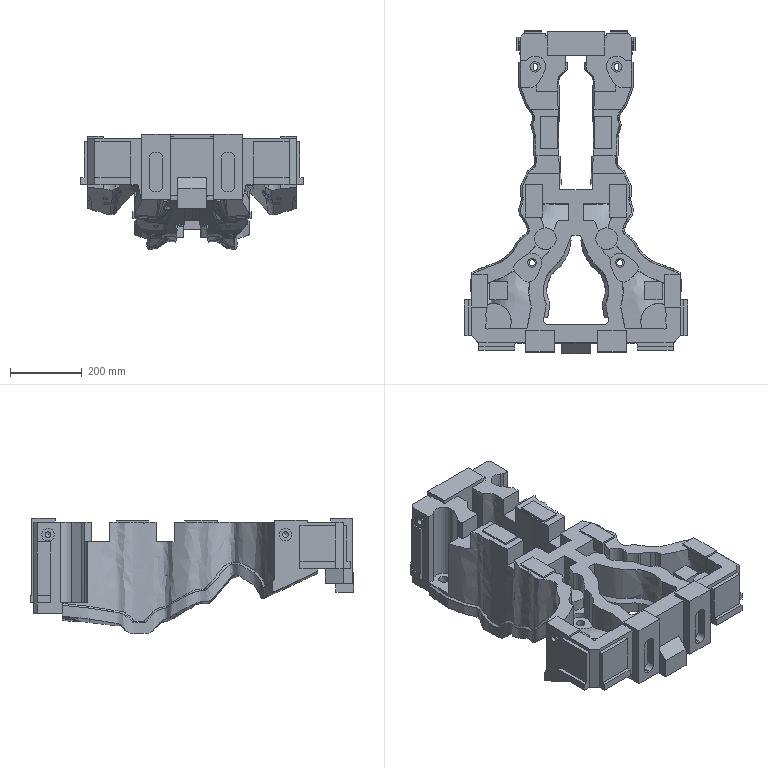Part | NX | features solid 2 | 1 solid | 1221 faces | box 620 x 900 x 320.126 mm | volume 41415893 mm3 | spline 872 | plane 275 | cylinder 68 | cone 6 | commonest cylinder face diameters 32 x18 60 x12 40 x7 11 x4 16 x4 35 x4